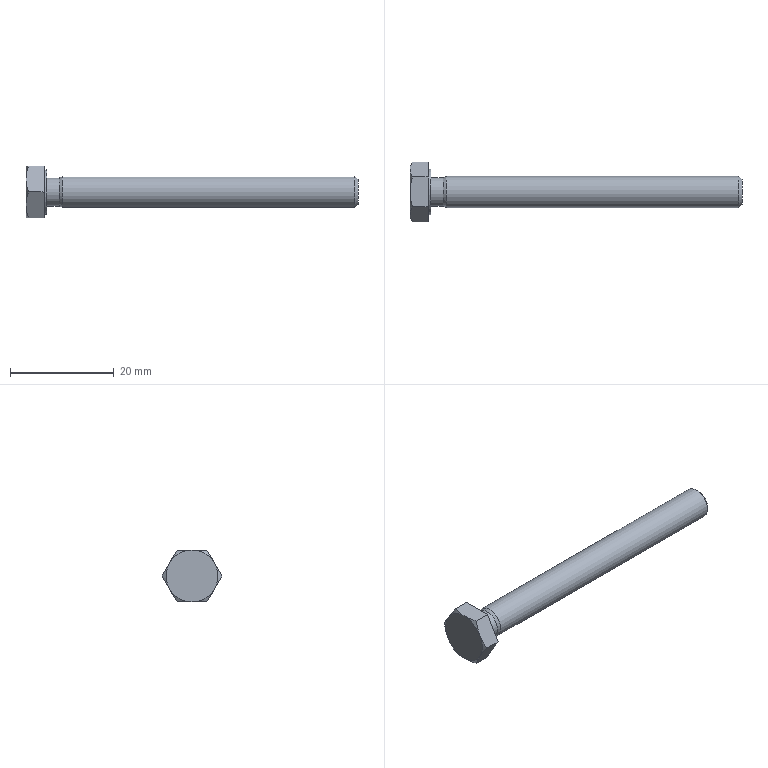Part | STEP file | DIN 933 - M6  x 60 | 1 solid | 21 faces | box 64 x 11.547 x 10 mm | volume 2012 mm3 | plane 10 | cone 8 | cylinder 3 | commonest cylinder face diameters 5.459 x1 6 x1 8.7 x1